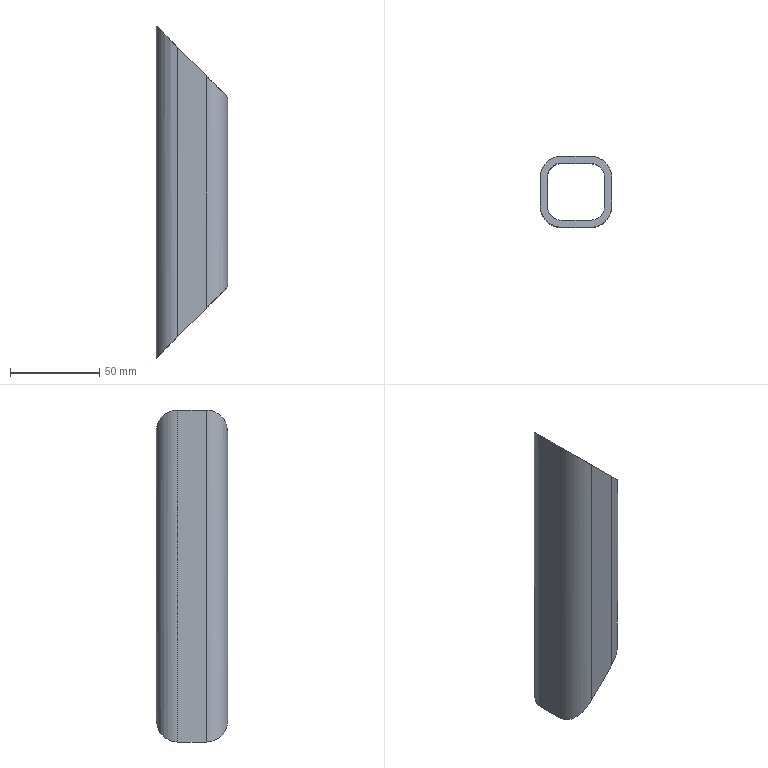Part | SolidWorks | features BaseBody 1 | 1 solid | 18 faces | box 40 x 40 x 185.969 mm | volume 74054 mm3 | plane 10 | cylinder 8 | commonest cylinder face diameters 16 x4 24 x4
STEP:
#1=CARTESIAN_POINT('',(-8.,-20.,173.969));
#2=VERTEX_POINT('',#1);
#3=CARTESIAN_POINT('',(-20.,-8.,185.969));
#4=VERTEX_POINT('',#3);
#5=CARTESIAN_POINT('',(-8.,-20.,173.969));
#6=CARTESIAN_POINT('',(-15.029,-20.,180.999));
#7=CARTESIAN_POINT('',(-20.,-15.029,185.969));
#8=CARTESIAN_POINT('',(-20.,-8.,185.969));
#9=(BOUNDED_CURVE()B_SPLINE_CURVE(3,(#5,#6,#7,#8),.UNSPECIFIED.,.F.,.F.)B_SPLINE_CURVE_WITH_KNOTS((4,4),(4.712,6.283),.UNSPECIFIED.)CURVE()GEOMETRIC_REPRESENTATION_ITEM()RATIONAL_B_SPLINE_CURVE((1.,0.8047,0.8047,1.))REPRESENTATION_ITEM(''));
#10=EDGE_CURVE('',#2,#4,#9,.T.);
#11=ORIENTED_EDGE('',*,*,#10,.T.);
#12=CARTESIAN_POINT('',(-20.,-8.,0.000000121));
#13=VERTEX_POINT('',#12);
#14=CARTESIAN_POINT('',(-20.,-8.,0.));
#15=DIRECTION('',(0.,0.,-1.));
#16=VECTOR('',#15,1000.);
#17=LINE('',#14,#16);
#18=EDGE_CURVE('',#4,#13,#17,.T.);
#19=ORIENTED_EDGE('',*,*,#18,.T.);
#20=CARTESIAN_POINT('',(-8.,-20.,12.));
#21=VERTEX_POINT('',#20);
#22=CARTESIAN_POINT('',(-20.,-8.,0.000000121));
#23=CARTESIAN_POINT('',(-20.,-15.029,0.000000241));
#24=CARTESIAN_POINT('',(-15.029,-20.,4.971));
#25=CARTESIAN_POINT('',(-8.,-20.,12.));
#26=(BOUNDED_CURVE()B_SPLINE_CURVE(3,(#22,#23,#24,#25),.UNSPECIFIED.,.F.,.F.)B_SPLINE_CURVE_WITH_KNOTS((4,4),(3.142,4.712),.UNSPECIFIED.)CURVE()GEOMETRIC_REPRESENTATION_ITEM()RATIONAL_B_SPLINE_CURVE((1.,0.8047,0.8047,1.))REPRESENTATION_ITEM(''));
#27=EDGE_CURVE('',#13,#21,#26,.T.);
#28=ORIENTED_EDGE('',*,*,#27,.T.);
#29=CARTESIAN_POINT('',(-8.,-20.,0.));
#30=DIRECTION('',(0.,0.,1.));
#31=VECTOR('',#30,1000.);
#32=LINE('',#29,#31);
#33=EDGE_CURVE('',#21,#2,#32,.T.);
#34=ORIENTED_EDGE('',*,*,#33,.T.);
#35=EDGE_LOOP('',(#11,#19,#28,#34));
#36=FACE_OUTER_BOUND('',#35,.T.);
#37=CARTESIAN_POINT('',(-8.,-8.,0.));
#38=DIRECTION('',(0.,0.,1.));
#39=DIRECTION('',(1.,0.,0.));
#40=AXIS2_PLACEMENT_3D('',#37,#38,#39);
#41=CYLINDRICAL_SURFACE('',#40,12.);
#42=ADVANCED_FACE('',(#36),#41,.T.);
#43=CARTESIAN_POINT('',(-20.,8.,0.000000121));
#44=VERTEX_POINT('',#43);
#45=CARTESIAN_POINT('',(-20.,-8.,0.));
#46=DIRECTION('',(0.,-1.,0.));
#47=VECTOR('',#46,1000.);
#48=LINE('',#45,#47);
#49=EDGE_CURVE('',#44,#13,#48,.T.);
#50=ORIENTED_EDGE('',*,*,#49,.T.);
#51=ORIENTED_EDGE('',*,*,#18,.F.);
#52=CARTESIAN_POINT('',(-20.,8.,185.969));
#53=VERTEX_POINT('',#52);
#54=CARTESIAN_POINT('',(-20.,-8.,185.969));
#55=DIRECTION('',(0.,1.,0.));
#56=VECTOR('',#55,1000.);
#57=LINE('',#54,#56);
#58=EDGE_CURVE('',#4,#53,#57,.T.);
#59=ORIENTED_EDGE('',*,*,#58,.T.);
#60=CARTESIAN_POINT('',(-20.,8.,0.));
#61=DIRECTION('',(0.,0.,-1.));
#62=VECTOR('',#61,1000.);
#63=LINE('',#60,#62);
#64=EDGE_CURVE('',#53,#44,#63,.T.);
#65=ORIENTED_EDGE('',*,*,#64,.T.);
#66=EDGE_LOOP('',(#50,#51,#59,#65));
#67=FACE_OUTER_BOUND('',#66,.T.);
#68=CARTESIAN_POINT('',(-20.,-8.,0.));
#69=DIRECTION('',(-1.,0.,0.));
#70=DIRECTION('',(0.,-1.,0.));
#71=AXIS2_PLACEMENT_3D('',#68,#69,#70);
#72=PLANE('',#71);
#73=ADVANCED_FACE('',(#67),#72,.T.);
#74=CARTESIAN_POINT('',(-16.,-8.,181.969));
#75=VERTEX_POINT('',#74);
#76=CARTESIAN_POINT('',(-8.,-16.,173.969));
#77=VERTEX_POINT('',#76);
#78=CARTESIAN_POINT('',(-16.,-8.,181.969));
#79=CARTESIAN_POINT('',(-16.,-12.686,181.969));
#80=CARTESIAN_POINT('',(-12.686,-16.,178.655));
#81=CARTESIAN_POINT('',(-8.,-16.,173.969));
#82=(BOUNDED_CURVE()B_SPLINE_CURVE(3,(#78,#79,#80,#81),.UNSPECIFIED.,.F.,.F.)B_SPLINE_CURVE_WITH_KNOTS((4,4),(0.,1.571),.UNSPECIFIED.)CURVE()GEOMETRIC_REPRESENTATION_ITEM()RATIONAL_B_SPLINE_CURVE((1.,0.8047,0.8047,1.))REPRESENTATION_ITEM(''));
#83=EDGE_CURVE('',#75,#77,#82,.T.);
#84=ORIENTED_EDGE('',*,*,#83,.F.);
#85=CARTESIAN_POINT('',(-16.,8.,181.969));
#86=VERTEX_POINT('',#85);
#87=CARTESIAN_POINT('',(-16.,0.,181.969));
#88=DIRECTION('',(0.,-1.,0.));
#89=VECTOR('',#88,1000.);
#90=LINE('',#87,#89);
#91=EDGE_CURVE('',#86,#75,#90,.T.);
#92=ORIENTED_EDGE('',*,*,#91,.F.);
#93=CARTESIAN_POINT('',(-8.,16.,173.969));
#94=VERTEX_POINT('',#93);
#95=CARTESIAN_POINT('',(-8.,16.,173.969));
#96=CARTESIAN_POINT('',(-12.686,16.,178.655));
#97=CARTESIAN_POINT('',(-16.,12.686,181.969));
#98=CARTESIAN_POINT('',(-16.,8.,181.969));
#99=(BOUNDED_CURVE()B_SPLINE_CURVE(3,(#95,#96,#97,#98),.UNSPECIFIED.,.F.,.F.)B_SPLINE_CURVE_WITH_KNOTS((4,4),(4.712,6.283),.UNSPECIFIED.)CURVE()GEOMETRIC_REPRESENTATION_ITEM()RATIONAL_B_SPLINE_CURVE((1.,0.8047,0.8047,1.))REPRESENTATION_ITEM(''));
#100=EDGE_CURVE('',#94,#86,#99,.T.);
#101=ORIENTED_EDGE('',*,*,#100,.F.);
#102=CARTESIAN_POINT('',(8.,16.,157.969));
#103=VERTEX_POINT('',#102);
#104=CARTESIAN_POINT('',(82.985,16.,82.985));
#105=DIRECTION('',(-0.7071,0.,0.7071));
#106=VECTOR('',#105,1000.);
#107=LINE('',#104,#106);
#108=EDGE_CURVE('',#103,#94,#107,.T.);
#109=ORIENTED_EDGE('',*,*,#108,.F.);
#110=CARTESIAN_POINT('',(16.,8.,149.969));
#111=VERTEX_POINT('',#110);
#112=CARTESIAN_POINT('',(16.,8.,149.969));
#113=CARTESIAN_POINT('',(16.,12.686,149.969));
#114=CARTESIAN_POINT('',(12.686,16.,153.283));
#115=CARTESIAN_POINT('',(8.,16.,157.969));
#116=(BOUNDED_CURVE()B_SPLINE_CURVE(3,(#112,#113,#114,#115),.UNSPECIFIED.,.F.,.F.)B_SPLINE_CURVE_WITH_KNOTS((4,4),(3.142,4.712),.UNSPECIFIED.)CURVE()GEOMETRIC_REPRESENTATION_ITEM()RATIONAL_B_SPLINE_CURVE((1.,0.8047,0.8047,1.))REPRESENTATION_ITEM(''));
#117=EDGE_CURVE('',#111,#103,#116,.T.);
#118=ORIENTED_EDGE('',*,*,#117,.F.);
#119=CARTESIAN_POINT('',(16.,-8.,149.969));
#120=VERTEX_POINT('',#119);
#121=CARTESIAN_POINT('',(16.,0.,149.969));
#122=DIRECTION('',(0.,1.,0.));
#123=VECTOR('',#122,1000.);
#124=LINE('',#121,#123);
#125=EDGE_CURVE('',#120,#111,#124,.T.);
#126=ORIENTED_EDGE('',*,*,#125,.F.);
#127=CARTESIAN_POINT('',(8.,-16.,157.969));
#128=VERTEX_POINT('',#127);
#129=CARTESIAN_POINT('',(8.,-16.,157.969));
#130=CARTESIAN_POINT('',(12.686,-16.,153.283));
#131=CARTESIAN_POINT('',(16.,-12.686,149.969));
#132=CARTESIAN_POINT('',(16.,-8.,149.969));
#133=(BOUNDED_CURVE()B_SPLINE_CURVE(3,(#129,#130,#131,#132),.UNSPECIFIED.,.F.,.F.)B_SPLINE_CURVE_WITH_KNOTS((4,4),(1.571,3.142),.UNSPECIFIED.)CURVE()GEOMETRIC_REPRESENTATION_ITEM()RATIONAL_B_SPLINE_CURVE((1.,0.8047,0.8047,1.))REPRESENTATION_ITEM(''));
#134=EDGE_CURVE('',#128,#120,#133,.T.);
#135=ORIENTED_EDGE('',*,*,#134,.F.);
#136=CARTESIAN_POINT('',(82.985,-16.,82.985));
#137=DIRECTION('',(0.7071,0.,-0.7071));
#138=VECTOR('',#137,1000.);
#139=LINE('',#136,#138);
#140=EDGE_CURVE('',#77,#128,#139,.T.);
#141=ORIENTED_EDGE('',*,*,#140,.F.);
#142=EDGE_LOOP('',(#84,#92,#101,#109,#118,#126,#135,#141));
#143=FACE_BOUND('',#142,.T.);
#144=CARTESIAN_POINT('',(8.,20.,157.969));
#145=VERTEX_POINT('',#144);
#146=CARTESIAN_POINT('',(20.,8.,145.969));
#147=VERTEX_POINT('',#146);
#148=CARTESIAN_POINT('',(8.,20.,157.969));
#149=CARTESIAN_POINT('',(15.029,20.,150.94));
#150=CARTESIAN_POINT('',(20.,15.029,145.969));
#151=CARTESIAN_POINT('',(20.,8.,145.969));
#152=(BOUNDED_CURVE()B_SPLINE_CURVE(3,(#148,#149,#150,#151),.UNSPECIFIED.,.F.,.F.)B_SPLINE_CURVE_WITH_KNOTS((4,4),(1.571,3.142),.UNSPECIFIED.)CURVE()GEOMETRIC_REPRESENTATION_ITEM()RATIONAL_B_SPLINE_CURVE((1.,0.8047,0.8047,1.))REPRESENTATION_ITEM(''));
#153=EDGE_CURVE('',#145,#147,#152,.T.);
#154=ORIENTED_EDGE('',*,*,#153,.F.);
#155=CARTESIAN_POINT('',(-8.,20.,173.969));
#156=VERTEX_POINT('',#155);
#157=CARTESIAN_POINT('',(82.985,20.,82.985));
#158=DIRECTION('',(0.7071,0.,-0.7071));
#159=VECTOR('',#158,1000.);
#160=LINE('',#157,#159);
#161=EDGE_CURVE('',#156,#145,#160,.T.);
#162=ORIENTED_EDGE('',*,*,#161,.F.);
#163=CARTESIAN_POINT('',(-20.,8.,185.969));
#164=CARTESIAN_POINT('',(-20.,15.029,185.969));
#165=CARTESIAN_POINT('',(-15.029,20.,180.999));
#166=CARTESIAN_POINT('',(-8.,20.,173.969));
#167=(BOUNDED_CURVE()B_SPLINE_CURVE(3,(#163,#164,#165,#166),.UNSPECIFIED.,.F.,.F.)B_SPLINE_CURVE_WITH_KNOTS((4,4),(0.,1.571),.UNSPECIFIED.)CURVE()GEOMETRIC_REPRESENTATION_ITEM()RATIONAL_B_SPLINE_CURVE((1.,0.8047,0.8047,1.))REPRESENTATION_ITEM(''));
#168=EDGE_CURVE('',#53,#156,#167,.T.);
#169=ORIENTED_EDGE('',*,*,#168,.F.);
#170=ORIENTED_EDGE('',*,*,#58,.F.);
#171=ORIENTED_EDGE('',*,*,#10,.F.);
#172=CARTESIAN_POINT('',(8.,-20.,157.969));
#173=VERTEX_POINT('',#172);
#174=CARTESIAN_POINT('',(82.985,-20.,82.985));
#175=DIRECTION('',(-0.7071,0.,0.7071));
#176=VECTOR('',#175,1000.);
#177=LINE('',#174,#176);
#178=EDGE_CURVE('',#173,#2,#177,.T.);
#179=ORIENTED_EDGE('',*,*,#178,.F.);
#180=CARTESIAN_POINT('',(20.,-8.,145.969));
#181=VERTEX_POINT('',#180);
#182=CARTESIAN_POINT('',(20.,-8.,145.969));
#183=CARTESIAN_POINT('',(20.,-15.029,145.969));
#184=CARTESIAN_POINT('',(15.029,-20.,150.94));
#185=CARTESIAN_POINT('',(8.,-20.,157.969));
#186=(BOUNDED_CURVE()B_SPLINE_CURVE(3,(#182,#183,#184,#185),.UNSPECIFIED.,.F.,.F.)B_SPLINE_CURVE_WITH_KNOTS((4,4),(3.142,4.712),.UNSPECIFIED.)CURVE()GEOMETRIC_REPRESENTATION_ITEM()RATIONAL_B_SPLINE_CURVE((1.,0.8047,0.8047,1.))REPRESENTATION_ITEM(''));
#187=EDGE_CURVE('',#181,#173,#186,.T.);
#188=ORIENTED_EDGE('',*,*,#187,.F.);
#189=CARTESIAN_POINT('',(20.,0.,145.969));
#190=DIRECTION('',(0.,-1.,0.));
#191=VECTOR('',#190,1000.);
#192=LINE('',#189,#191);
#193=EDGE_CURVE('',#147,#181,#192,.T.);
#194=ORIENTED_EDGE('',*,*,#193,.F.);
#195=EDGE_LOOP('',(#154,#162,#169,#170,#171,#179,#188,#194));
#196=FACE_OUTER_BOUND('',#195,.T.);
#197=CARTESIAN_POINT('',(82.985,0.,82.985));
#198=DIRECTION('',(-0.7071,0.,-0.7071));
#199=DIRECTION('',(-0.7071,0.,0.7071));
#200=AXIS2_PLACEMENT_3D('',#197,#198,#199);
#201=PLANE('',#200);
#202=ADVANCED_FACE('',(#143,#196),#201,.F.);
#203=ORIENTED_EDGE('',*,*,#178,.T.);
#204=ORIENTED_EDGE('',*,*,#33,.F.);
#205=CARTESIAN_POINT('',(8.,-20.,28.));
#206=VERTEX_POINT('',#205);
#207=CARTESIAN_POINT('',(-8.,-20.,12.));
#208=DIRECTION('',(0.7071,0.,0.7071));
#209=VECTOR('',#208,1000.);
#210=LINE('',#207,#209);
#211=EDGE_CURVE('',#21,#206,#210,.T.);
#212=ORIENTED_EDGE('',*,*,#211,.T.);
#213=CARTESIAN_POINT('',(8.,-20.,0.));
#214=DIRECTION('',(0.,0.,1.));
#215=VECTOR('',#214,1000.);
#216=LINE('',#213,#215);
#217=EDGE_CURVE('',#206,#173,#216,.T.);
#218=ORIENTED_EDGE('',*,*,#217,.T.);
#219=EDGE_LOOP('',(#203,#204,#212,#218));
#220=FACE_OUTER_BOUND('',#219,.T.);
#221=CARTESIAN_POINT('',(8.,-20.,0.));
#222=DIRECTION('',(0.,-1.,0.));
#223=DIRECTION('',(1.,0.,0.));
#224=AXIS2_PLACEMENT_3D('',#221,#222,#223);
#225=PLANE('',#224);
#226=ADVANCED_FACE('',(#220),#225,.T.);
#227=CARTESIAN_POINT('',(-16.,8.,4.));
#228=VERTEX_POINT('',#227);
#229=CARTESIAN_POINT('',(-8.,16.,12.));
#230=VERTEX_POINT('',#229);
#231=CARTESIAN_POINT('',(-16.,8.,4.));
#232=CARTESIAN_POINT('',(-16.,12.686,4.));
#233=CARTESIAN_POINT('',(-12.686,16.,7.314));
#234=CARTESIAN_POINT('',(-8.,16.,12.));
#235=(BOUNDED_CURVE()B_SPLINE_CURVE(3,(#231,#232,#233,#234),.UNSPECIFIED.,.F.,.F.)B_SPLINE_CURVE_WITH_KNOTS((4,4),(3.142,4.712),.UNSPECIFIED.)CURVE()GEOMETRIC_REPRESENTATION_ITEM()RATIONAL_B_SPLINE_CURVE((1.,0.8047,0.8047,1.))REPRESENTATION_ITEM(''));
#236=EDGE_CURVE('',#228,#230,#235,.T.);
#237=ORIENTED_EDGE('',*,*,#236,.F.);
#238=CARTESIAN_POINT('',(-16.,-8.,4.));
#239=VERTEX_POINT('',#238);
#240=CARTESIAN_POINT('',(-16.,0.,4.));
#241=DIRECTION('',(0.,1.,0.));
#242=VECTOR('',#241,1000.);
#243=LINE('',#240,#242);
#244=EDGE_CURVE('',#239,#228,#243,.T.);
#245=ORIENTED_EDGE('',*,*,#244,.F.);
#246=CARTESIAN_POINT('',(-8.,-16.,12.));
#247=VERTEX_POINT('',#246);
#248=CARTESIAN_POINT('',(-8.,-16.,12.));
#249=CARTESIAN_POINT('',(-12.686,-16.,7.314));
#250=CARTESIAN_POINT('',(-16.,-12.686,4.));
#251=CARTESIAN_POINT('',(-16.,-8.,4.));
#252=(BOUNDED_CURVE()B_SPLINE_CURVE(3,(#248,#249,#250,#251),.UNSPECIFIED.,.F.,.F.)B_SPLINE_CURVE_WITH_KNOTS((4,4),(1.571,3.142),.UNSPECIFIED.)CURVE()GEOMETRIC_REPRESENTATION_ITEM()RATIONAL_B_SPLINE_CURVE((1.,0.8047,0.8047,1.))REPRESENTATION_ITEM(''));
#253=EDGE_CURVE('',#247,#239,#252,.T.);
#254=ORIENTED_EDGE('',*,*,#253,.F.);
#255=CARTESIAN_POINT('',(8.,-16.,28.));
#256=VERTEX_POINT('',#255);
#257=CARTESIAN_POINT('',(-10.,-16.,10.));
#258=DIRECTION('',(-0.7071,0.,-0.7071));
#259=VECTOR('',#258,1000.);
#260=LINE('',#257,#259);
#261=EDGE_CURVE('',#256,#247,#260,.T.);
#262=ORIENTED_EDGE('',*,*,#261,.F.);
#263=CARTESIAN_POINT('',(16.,-8.,36.));
#264=VERTEX_POINT('',#263);
#265=CARTESIAN_POINT('',(16.,-8.,36.));
#266=CARTESIAN_POINT('',(16.,-12.686,36.));
#267=CARTESIAN_POINT('',(12.686,-16.,32.686));
#268=CARTESIAN_POINT('',(8.,-16.,28.));
#269=(BOUNDED_CURVE()B_SPLINE_CURVE(3,(#265,#266,#267,#268),.UNSPECIFIED.,.F.,.F.)B_SPLINE_CURVE_WITH_KNOTS((4,4),(0.,1.571),.UNSPECIFIED.)CURVE()GEOMETRIC_REPRESENTATION_ITEM()RATIONAL_B_SPLINE_CURVE((1.,0.8047,0.8047,1.))REPRESENTATION_ITEM(''));
#270=EDGE_CURVE('',#264,#256,#269,.T.);
#271=ORIENTED_EDGE('',*,*,#270,.F.);
#272=CARTESIAN_POINT('',(16.,8.,36.));
#273=VERTEX_POINT('',#272);
#274=CARTESIAN_POINT('',(16.,0.,36.));
#275=DIRECTION('',(0.,-1.,0.));
#276=VECTOR('',#275,1000.);
#277=LINE('',#274,#276);
#278=EDGE_CURVE('',#273,#264,#277,.T.);
#279=ORIENTED_EDGE('',*,*,#278,.F.);
#280=CARTESIAN_POINT('',(8.,16.,28.));
#281=VERTEX_POINT('',#280);
#282=CARTESIAN_POINT('',(8.,16.,28.));
#283=CARTESIAN_POINT('',(12.686,16.,32.686));
#284=CARTESIAN_POINT('',(16.,12.686,36.));
#285=CARTESIAN_POINT('',(16.,8.,36.));
#286=(BOUNDED_CURVE()B_SPLINE_CURVE(3,(#282,#283,#284,#285),.UNSPECIFIED.,.F.,.F.)B_SPLINE_CURVE_WITH_KNOTS((4,4),(4.712,6.283),.UNSPECIFIED.)CURVE()GEOMETRIC_REPRESENTATION_ITEM()RATIONAL_B_SPLINE_CURVE((1.,0.8047,0.8047,1.))REPRESENTATION_ITEM(''));
#287=EDGE_CURVE('',#281,#273,#286,.T.);
#288=ORIENTED_EDGE('',*,*,#287,.F.);
#289=CARTESIAN_POINT('',(-10.,16.,10.));
#290=DIRECTION('',(0.7071,0.,0.7071));
#291=VECTOR('',#290,1000.);
#292=LINE('',#289,#291);
#293=EDGE_CURVE('',#230,#281,#292,.T.);
#294=ORIENTED_EDGE('',*,*,#293,.F.);
#295=EDGE_LOOP('',(#237,#245,#254,#262,#271,#279,#288,#294));
#296=FACE_BOUND('',#295,.T.);
#297=CARTESIAN_POINT('',(8.,20.,28.));
#298=VERTEX_POINT('',#297);
#299=CARTESIAN_POINT('',(-8.,20.,12.));
#300=VERTEX_POINT('',#299);
#301=CARTESIAN_POINT('',(-10.,20.,10.));
#302=DIRECTION('',(-0.7071,0.,-0.7071));
#303=VECTOR('',#302,1000.);
#304=LINE('',#301,#303);
#305=EDGE_CURVE('',#298,#300,#304,.T.);
#306=ORIENTED_EDGE('',*,*,#305,.F.);
#307=CARTESIAN_POINT('',(20.,8.,40.));
#308=VERTEX_POINT('',#307);
#309=CARTESIAN_POINT('',(20.,8.,40.));
#310=CARTESIAN_POINT('',(20.,15.029,40.));
#311=CARTESIAN_POINT('',(15.029,20.,35.029));
#312=CARTESIAN_POINT('',(8.,20.,28.));
#313=(BOUNDED_CURVE()B_SPLINE_CURVE(3,(#309,#310,#311,#312),.UNSPECIFIED.,.F.,.T.)B_SPLINE_CURVE_WITH_KNOTS((4,4),(0.,1.571),.UNSPECIFIED.)CURVE()GEOMETRIC_REPRESENTATION_ITEM()RATIONAL_B_SPLINE_CURVE((1.,0.8047,0.8047,1.))REPRESENTATION_ITEM(''));
#314=EDGE_CURVE('',#308,#298,#313,.T.);
#315=ORIENTED_EDGE('',*,*,#314,.F.);
#316=CARTESIAN_POINT('',(20.,-8.,40.));
#317=VERTEX_POINT('',#316);
#318=CARTESIAN_POINT('',(20.,0.,40.));
#319=DIRECTION('',(0.,1.,0.));
#320=VECTOR('',#319,1000.);
#321=LINE('',#318,#320);
#322=EDGE_CURVE('',#317,#308,#321,.T.);
#323=ORIENTED_EDGE('',*,*,#322,.F.);
#324=CARTESIAN_POINT('',(8.,-20.,28.));
#325=CARTESIAN_POINT('',(15.029,-20.,35.029));
#326=CARTESIAN_POINT('',(20.,-15.029,40.));
#327=CARTESIAN_POINT('',(20.,-8.,40.));
#328=(BOUNDED_CURVE()B_SPLINE_CURVE(3,(#324,#325,#326,#327),.UNSPECIFIED.,.F.,.F.)B_SPLINE_CURVE_WITH_KNOTS((4,4),(4.712,6.283),.UNSPECIFIED.)CURVE()GEOMETRIC_REPRESENTATION_ITEM()RATIONAL_B_SPLINE_CURVE((1.,0.8047,0.8047,1.))REPRESENTATION_ITEM(''));
#329=EDGE_CURVE('',#206,#317,#328,.T.);
#330=ORIENTED_EDGE('',*,*,#329,.F.);
#331=ORIENTED_EDGE('',*,*,#211,.F.);
#332=ORIENTED_EDGE('',*,*,#27,.F.);
#333=ORIENTED_EDGE('',*,*,#49,.F.);
#334=CARTESIAN_POINT('',(-8.,20.,12.));
#335=CARTESIAN_POINT('',(-15.029,20.,4.971));
#336=CARTESIAN_POINT('',(-20.,15.029,0.000000241));
#337=CARTESIAN_POINT('',(-20.,8.,0.000000121));
#338=(BOUNDED_CURVE()B_SPLINE_CURVE(3,(#334,#335,#336,#337),.UNSPECIFIED.,.F.,.F.)B_SPLINE_CURVE_WITH_KNOTS((4,4),(1.571,3.142),.UNSPECIFIED.)CURVE()GEOMETRIC_REPRESENTATION_ITEM()RATIONAL_B_SPLINE_CURVE((1.,0.8047,0.8047,1.))REPRESENTATION_ITEM(''));
#339=EDGE_CURVE('',#300,#44,#338,.T.);
#340=ORIENTED_EDGE('',*,*,#339,.F.);
#341=EDGE_LOOP('',(#306,#315,#323,#330,#331,#332,#333,#340));
#342=FACE_OUTER_BOUND('',#341,.T.);
#343=CARTESIAN_POINT('',(-10.,0.,10.));
#344=DIRECTION('',(-0.7071,0.,0.7071));
#345=DIRECTION('',(0.7071,0.,0.7071));
#346=AXIS2_PLACEMENT_3D('',#343,#344,#345);
#347=PLANE('',#346);
#348=ADVANCED_FACE('',(#296,#342),#347,.F.);
#349=ORIENTED_EDGE('',*,*,#168,.T.);
#350=CARTESIAN_POINT('',(-8.,20.,0.));
#351=DIRECTION('',(0.,0.,-1.));
#352=VECTOR('',#351,1000.);
#353=LINE('',#350,#352);
#354=EDGE_CURVE('',#156,#300,#353,.T.);
#355=ORIENTED_EDGE('',*,*,#354,.T.);
#356=ORIENTED_EDGE('',*,*,#339,.T.);
#357=ORIENTED_EDGE('',*,*,#64,.F.);
#358=EDGE_LOOP('',(#349,#355,#356,#357));
#359=FACE_OUTER_BOUND('',#358,.T.);
#360=CARTESIAN_POINT('',(-8.,8.,0.));
#361=DIRECTION('',(0.,0.,1.));
#362=DIRECTION('',(1.,0.,0.));
#363=AXIS2_PLACEMENT_3D('',#360,#361,#362);
#364=CYLINDRICAL_SURFACE('',#363,12.);
#365=ADVANCED_FACE('',(#359),#364,.T.);
#366=CARTESIAN_POINT('',(-8.,-16.,0.));
#367=DIRECTION('',(0.,0.,-1.));
#368=VECTOR('',#367,1000.);
#369=LINE('',#366,#368);
#370=EDGE_CURVE('',#77,#247,#369,.T.);
#371=ORIENTED_EDGE('',*,*,#370,.F.);
#372=ORIENTED_EDGE('',*,*,#140,.T.);
#373=CARTESIAN_POINT('',(8.,-16.,0.));
#374=DIRECTION('',(0.,0.,1.));
#375=VECTOR('',#374,1000.);
#376=LINE('',#373,#375);
#377=EDGE_CURVE('',#256,#128,#376,.T.);
#378=ORIENTED_EDGE('',*,*,#377,.F.);
#379=ORIENTED_EDGE('',*,*,#261,.T.);
#380=EDGE_LOOP('',(#371,#372,#378,#379));
#381=FACE_OUTER_BOUND('',#380,.T.);
#382=CARTESIAN_POINT('',(8.,-16.,0.));
#383=DIRECTION('',(0.,-1.,0.));
#384=DIRECTION('',(1.,0.,0.));
#385=AXIS2_PLACEMENT_3D('',#382,#383,#384);
#386=PLANE('',#385);
#387=ADVANCED_FACE('',(#381),#386,.F.);
#388=CARTESIAN_POINT('',(-16.,-8.,0.));
#389=DIRECTION('',(0.,0.,-1.));
#390=VECTOR('',#389,1000.);
#391=LINE('',#388,#390);
#392=EDGE_CURVE('',#75,#239,#391,.T.);
#393=ORIENTED_EDGE('',*,*,#392,.F.);
#394=ORIENTED_EDGE('',*,*,#83,.T.);
#395=ORIENTED_EDGE('',*,*,#370,.T.);
#396=ORIENTED_EDGE('',*,*,#253,.T.);
#397=EDGE_LOOP('',(#393,#394,#395,#396));
#398=FACE_OUTER_BOUND('',#397,.T.);
#399=CARTESIAN_POINT('',(-8.,-8.,0.));
#400=DIRECTION('',(0.,0.,1.));
#401=DIRECTION('',(1.,0.,0.));
#402=AXIS2_PLACEMENT_3D('',#399,#400,#401);
#403=CYLINDRICAL_SURFACE('',#402,8.);
#404=ADVANCED_FACE('',(#398),#403,.F.);
#405=CARTESIAN_POINT('',(-16.,8.,0.));
#406=DIRECTION('',(0.,0.,-1.));
#407=VECTOR('',#406,1000.);
#408=LINE('',#405,#407);
#409=EDGE_CURVE('',#86,#228,#408,.T.);
#410=ORIENTED_EDGE('',*,*,#409,.F.);
#411=ORIENTED_EDGE('',*,*,#91,.T.);
#412=ORIENTED_EDGE('',*,*,#392,.T.);
#413=ORIENTED_EDGE('',*,*,#244,.T.);
#414=EDGE_LOOP('',(#410,#411,#412,#413));
#415=FACE_OUTER_BOUND('',#414,.T.);
#416=CARTESIAN_POINT('',(-16.,-8.,0.));
#417=DIRECTION('',(-1.,0.,0.));
#418=DIRECTION('',(0.,-1.,0.));
#419=AXIS2_PLACEMENT_3D('',#416,#417,#418);
#420=PLANE('',#419);
#421=ADVANCED_FACE('',(#415),#420,.F.);
#422=CARTESIAN_POINT('',(-8.,16.,0.));
#423=DIRECTION('',(0.,0.,-1.));
#424=VECTOR('',#423,1000.);
#425=LINE('',#422,#424);
#426=EDGE_CURVE('',#94,#230,#425,.T.);
#427=ORIENTED_EDGE('',*,*,#426,.F.);
#428=ORIENTED_EDGE('',*,*,#100,.T.);
#429=ORIENTED_EDGE('',*,*,#409,.T.);
#430=ORIENTED_EDGE('',*,*,#236,.T.);
#431=EDGE_LOOP('',(#427,#428,#429,#430));
#432=FACE_OUTER_BOUND('',#431,.T.);
#433=CARTESIAN_POINT('',(-8.,8.,0.));
#434=DIRECTION('',(0.,0.,1.));
#435=DIRECTION('',(1.,0.,0.));
#436=AXIS2_PLACEMENT_3D('',#433,#434,#435);
#437=CYLINDRICAL_SURFACE('',#436,8.);
#438=ADVANCED_FACE('',(#432),#437,.F.);
#439=CARTESIAN_POINT('',(8.,16.,0.));
#440=DIRECTION('',(0.,0.,-1.));
#441=VECTOR('',#440,1000.);
#442=LINE('',#439,#441);
#443=EDGE_CURVE('',#103,#281,#442,.T.);
#444=ORIENTED_EDGE('',*,*,#443,.F.);
#445=ORIENTED_EDGE('',*,*,#108,.T.);
#446=ORIENTED_EDGE('',*,*,#426,.T.);
#447=ORIENTED_EDGE('',*,*,#293,.T.);
#448=EDGE_LOOP('',(#444,#445,#446,#447));
#449=FACE_OUTER_BOUND('',#448,.T.);
#450=CARTESIAN_POINT('',(-8.,16.,0.));
#451=DIRECTION('',(0.,1.,0.));
#452=DIRECTION('',(-1.,0.,0.));
#453=AXIS2_PLACEMENT_3D('',#450,#451,#452);
#454=PLANE('',#453);
#455=ADVANCED_FACE('',(#449),#454,.F.);
#456=CARTESIAN_POINT('',(16.,8.,0.));
#457=DIRECTION('',(0.,0.,-1.));
#458=VECTOR('',#457,1000.);
#459=LINE('',#456,#458);
#460=EDGE_CURVE('',#111,#273,#459,.T.);
#461=ORIENTED_EDGE('',*,*,#460,.F.);
#462=ORIENTED_EDGE('',*,*,#117,.T.);
#463=ORIENTED_EDGE('',*,*,#443,.T.);
#464=ORIENTED_EDGE('',*,*,#287,.T.);
#465=EDGE_LOOP('',(#461,#462,#463,#464));
#466=FACE_OUTER_BOUND('',#465,.T.);
#467=CARTESIAN_POINT('',(8.,8.,0.));
#468=DIRECTION('',(0.,0.,1.));
#469=DIRECTION('',(1.,0.,0.));
#470=AXIS2_PLACEMENT_3D('',#467,#468,#469);
#471=CYLINDRICAL_SURFACE('',#470,8.);
#472=ADVANCED_FACE('',(#466),#471,.F.);
#473=CARTESIAN_POINT('',(16.,-8.,0.));
#474=DIRECTION('',(0.,0.,-1.));
#475=VECTOR('',#474,1000.);
#476=LINE('',#473,#475);
#477=EDGE_CURVE('',#120,#264,#476,.T.);
#478=ORIENTED_EDGE('',*,*,#477,.F.);
#479=ORIENTED_EDGE('',*,*,#125,.T.);
#480=ORIENTED_EDGE('',*,*,#460,.T.);
#481=ORIENTED_EDGE('',*,*,#278,.T.);
#482=EDGE_LOOP('',(#478,#479,#480,#481));
#483=FACE_OUTER_BOUND('',#482,.T.);
#484=CARTESIAN_POINT('',(16.,8.,0.));
#485=DIRECTION('',(1.,0.,0.));
#486=DIRECTION('',(0.,0.,-1.));
#487=AXIS2_PLACEMENT_3D('',#484,#485,#486);
#488=PLANE('',#487);
#489=ADVANCED_FACE('',(#483),#488,.F.);
#490=ORIENTED_EDGE('',*,*,#377,.T.);
#491=ORIENTED_EDGE('',*,*,#134,.T.);
#492=ORIENTED_EDGE('',*,*,#477,.T.);
#493=ORIENTED_EDGE('',*,*,#270,.T.);
#494=EDGE_LOOP('',(#490,#491,#492,#493));
#495=FACE_OUTER_BOUND('',#494,.T.);
#496=CARTESIAN_POINT('',(8.,-8.,0.));
#497=DIRECTION('',(0.,0.,1.));
#498=DIRECTION('',(1.,0.,0.));
#499=AXIS2_PLACEMENT_3D('',#496,#497,#498);
#500=CYLINDRICAL_SURFACE('',#499,8.);
#501=ADVANCED_FACE('',(#495),#500,.F.);
#502=ORIENTED_EDGE('',*,*,#193,.T.);
#503=CARTESIAN_POINT('',(20.,-8.,0.));
#504=DIRECTION('',(0.,0.,-1.));
#505=VECTOR('',#504,1000.);
#506=LINE('',#503,#505);
#507=EDGE_CURVE('',#181,#317,#506,.T.);
#508=ORIENTED_EDGE('',*,*,#507,.T.);
#509=ORIENTED_EDGE('',*,*,#322,.T.);
#510=CARTESIAN_POINT('',(20.,8.,0.));
#511=DIRECTION('',(0.,0.,1.));
#512=VECTOR('',#511,1000.);
#513=LINE('',#510,#512);
#514=EDGE_CURVE('',#308,#147,#513,.T.);
#515=ORIENTED_EDGE('',*,*,#514,.T.);
#516=EDGE_LOOP('',(#502,#508,#509,#515));
#517=FACE_OUTER_BOUND('',#516,.T.);
#518=CARTESIAN_POINT('',(20.,8.,0.));
#519=DIRECTION('',(1.,0.,0.));
#520=DIRECTION('',(0.,1.,0.));
#521=AXIS2_PLACEMENT_3D('',#518,#519,#520);
#522=PLANE('',#521);
#523=ADVANCED_FACE('',(#517),#522,.T.);
#524=ORIENTED_EDGE('',*,*,#153,.T.);
#525=ORIENTED_EDGE('',*,*,#514,.F.);
#526=ORIENTED_EDGE('',*,*,#314,.T.);
#527=CARTESIAN_POINT('',(8.,20.,0.));
#528=DIRECTION('',(0.,0.,1.));
#529=VECTOR('',#528,1000.);
#530=LINE('',#527,#529);
#531=EDGE_CURVE('',#298,#145,#530,.T.);
#532=ORIENTED_EDGE('',*,*,#531,.T.);
#533=EDGE_LOOP('',(#524,#525,#526,#532));
#534=FACE_OUTER_BOUND('',#533,.T.);
#535=CARTESIAN_POINT('',(8.,8.,0.));
#536=DIRECTION('',(0.,0.,1.));
#537=DIRECTION('',(1.,0.,0.));
#538=AXIS2_PLACEMENT_3D('',#535,#536,#537);
#539=CYLINDRICAL_SURFACE('',#538,12.);
#540=ADVANCED_FACE('',(#534),#539,.T.);
#541=ORIENTED_EDGE('',*,*,#161,.T.);
#542=ORIENTED_EDGE('',*,*,#531,.F.);
#543=ORIENTED_EDGE('',*,*,#305,.T.);
#544=ORIENTED_EDGE('',*,*,#354,.F.);
#545=EDGE_LOOP('',(#541,#542,#543,#544));
#546=FACE_OUTER_BOUND('',#545,.T.);
#547=CARTESIAN_POINT('',(-8.,20.,0.));
#548=DIRECTION('',(0.,1.,0.));
#549=DIRECTION('',(0.,0.,1.));
#550=AXIS2_PLACEMENT_3D('',#547,#548,#549);
#551=PLANE('',#550);
#552=ADVANCED_FACE('',(#546),#551,.T.);
#553=ORIENTED_EDGE('',*,*,#187,.T.);
#554=ORIENTED_EDGE('',*,*,#217,.F.);
#555=ORIENTED_EDGE('',*,*,#329,.T.);
#556=ORIENTED_EDGE('',*,*,#507,.F.);
#557=EDGE_LOOP('',(#553,#554,#555,#556));
#558=FACE_OUTER_BOUND('',#557,.T.);
#559=CARTESIAN_POINT('',(8.,-8.,0.));
#560=DIRECTION('',(0.,0.,1.));
#561=DIRECTION('',(1.,0.,0.));
#562=AXIS2_PLACEMENT_3D('',#559,#560,#561);
#563=CYLINDRICAL_SURFACE('',#562,12.);
#564=ADVANCED_FACE('',(#558),#563,.T.);
#565=CLOSED_SHELL('',(#42,#73,#202,#226,#348,#365,#387,#404,#421,#438,#455,#472,#489,#501,#523,#540,#552,#564));
#566=MANIFOLD_SOLID_BREP('',#565);
#567=CARTESIAN_POINT('',(0.,0.,0.));
#568=DIRECTION('',(0.,0.,1.));
#569=DIRECTION('',(1.,0.,0.));
#570=AXIS2_PLACEMENT_3D('',#567,#568,#569);
#571=(LENGTH_UNIT()NAMED_UNIT(*)SI_UNIT(.MILLI.,.METRE.));
#572=UNCERTAINTY_MEASURE_WITH_UNIT(LENGTH_MEASURE(0.00001),#571,'','');
#573=(NAMED_UNIT(*)PLANE_ANGLE_UNIT()SI_UNIT($,.RADIAN.));
#574=(NAMED_UNIT(*)SI_UNIT($,.STERADIAN.)SOLID_ANGLE_UNIT());
#575=(GEOMETRIC_REPRESENTATION_CONTEXT(3)GLOBAL_UNCERTAINTY_ASSIGNED_CONTEXT((#572))GLOBAL_UNIT_ASSIGNED_CONTEXT((#571,#573,#574))REPRESENTATION_CONTEXT('',''));
#576=ADVANCED_BREP_SHAPE_REPRESENTATION('',(#566,#570),#575);